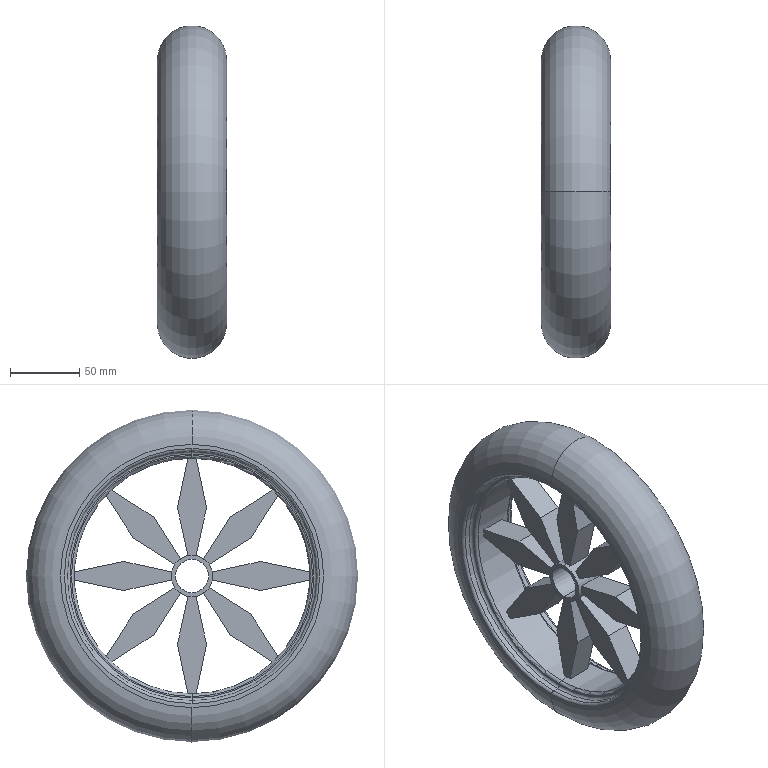Part | SolidWorks | features ICE 3, CirPattern 1, Fillet 1, Revolution 1 | 1 solid | 78 faces | box 50 x 239.862 x 239.862 mm | volume 1028496 mm3 | plane 54 | torus 14 | cylinder 10 | commonest cylinder face diameters 180 x4 24 x2 30 x2 170 x2